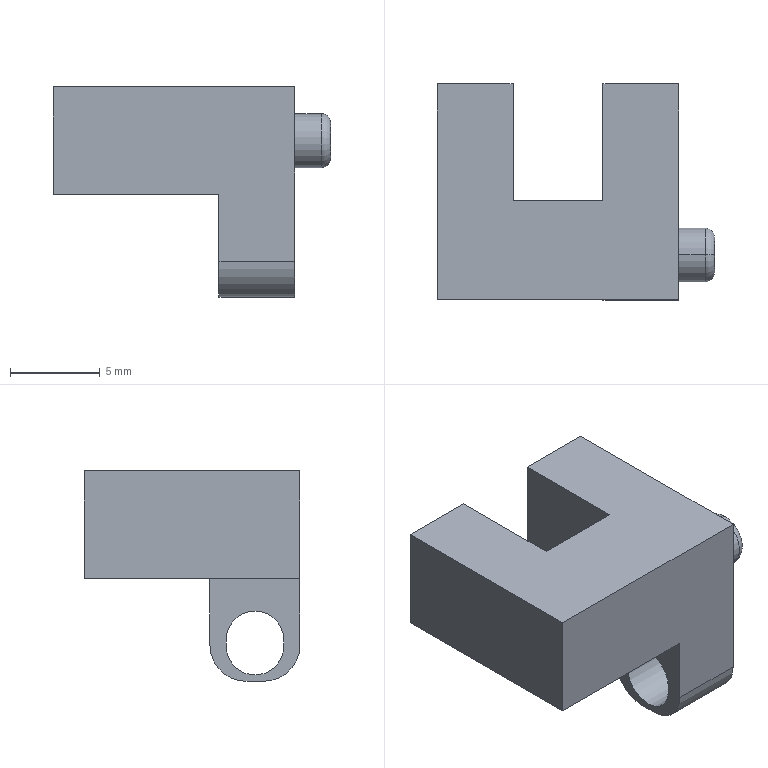Part | STEP file | 001-008-PM-F25 (Panasonic) | 1 solid | 25 faces | box 15.4 x 12 x 11.7 mm | volume 857.476 mm3 | plane 16 | cylinder 7 | torus 2 | commonest cylinder face diameters 3.2 x3 3 x2 4 x2